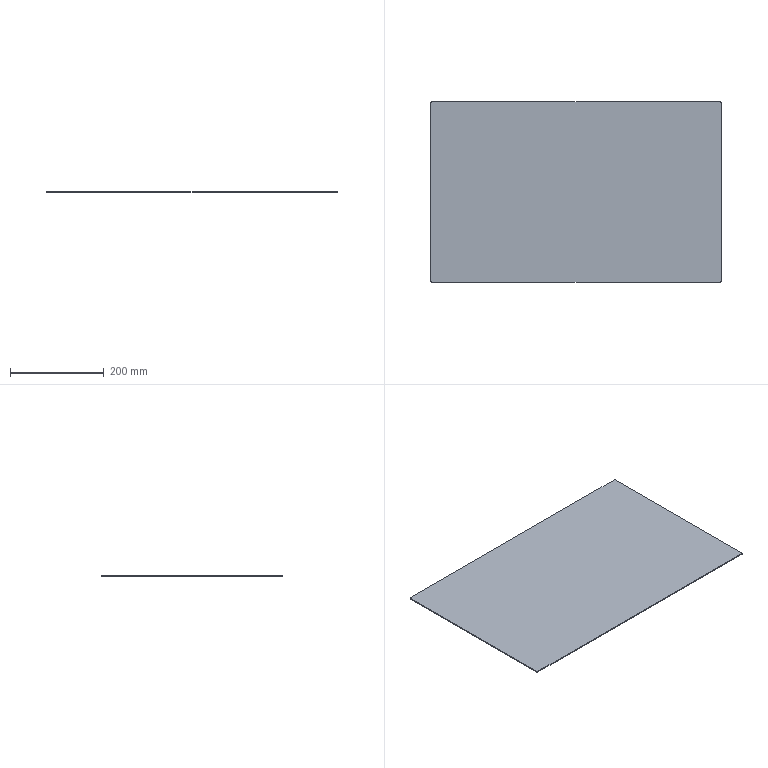Part | STEP file | Kanban base plate | 1 solid | 10 faces | box 620 x 386 x 2 mm | volume 478633 mm3 | plane 6 | cylinder 4 | commonest cylinder face diameters 4 x4
STEP:
#1=CARTESIAN_POINT('',(0.,0.,0.));
#2=DIRECTION('',(0.,0.,1.));
#3=DIRECTION('',(1.,0.,0.));
#4=AXIS2_PLACEMENT_3D('',#1,#2,#3);
#5=CARTESIAN_POINT('',(310.,-191.,2.));
#6=VERTEX_POINT('',#5);
#7=CARTESIAN_POINT('',(310.,191.,2.));
#8=VERTEX_POINT('',#7);
#9=CARTESIAN_POINT('',(310.,193.,2.));
#10=DIRECTION('',(0.,1.,0.));
#11=VECTOR('',#10,1.);
#12=LINE('',#9,#11);
#13=CARTESIAN_POINT('',(310.,193.,2.));
#14=DIRECTION('',(-1.,0.,0.));
#15=DIRECTION('',(0.,0.,1.));
#16=AXIS2_PLACEMENT_3D('',#13,#14,#15);
#17=PLANE('',#16);
#18=CARTESIAN_POINT('',(0.,0.));
#19=DIRECTION('',(0.,1.));
#20=VECTOR('',#19,1.);
#21=LINE('',#18,#20);
#22=(GEOMETRIC_REPRESENTATION_CONTEXT(2)PARAMETRIC_REPRESENTATION_CONTEXT()REPRESENTATION_CONTEXT('',''));
#23=DEFINITIONAL_REPRESENTATION('',(#21),#22);
#24=PCURVE('',#17,#23);
#25=CARTESIAN_POINT('',(0.,0.,2.));
#26=DIRECTION('',(0.,0.,1.));
#27=DIRECTION('',(1.,0.,0.));
#28=AXIS2_PLACEMENT_3D('',#25,#26,#27);
#29=PLANE('',#28);
#30=CARTESIAN_POINT('',(310.,193.));
#31=DIRECTION('',(0.,1.));
#32=VECTOR('',#31,1.);
#33=LINE('',#30,#32);
#34=(GEOMETRIC_REPRESENTATION_CONTEXT(2)PARAMETRIC_REPRESENTATION_CONTEXT()REPRESENTATION_CONTEXT('',''));
#35=DEFINITIONAL_REPRESENTATION('',(#33),#34);
#36=PCURVE('',#29,#35);
#37=SURFACE_CURVE('',#12,(#24,#36),.PCURVE_S1.);
#38=EDGE_CURVE('',#6,#8,#37,.T.);
#39=ORIENTED_EDGE('',*,*,#38,.F.);
#40=CARTESIAN_POINT('',(310.,-191.,0.));
#41=VERTEX_POINT('',#40);
#42=CARTESIAN_POINT('',(310.,-191.,2.));
#43=DIRECTION('',(0.,0.,-1.));
#44=VECTOR('',#43,1.);
#45=LINE('',#42,#44);
#46=CARTESIAN_POINT('',(0.,-384.));
#47=DIRECTION('',(-1.,0.));
#48=VECTOR('',#47,1.);
#49=LINE('',#46,#48);
#50=(GEOMETRIC_REPRESENTATION_CONTEXT(2)PARAMETRIC_REPRESENTATION_CONTEXT()REPRESENTATION_CONTEXT('',''));
#51=DEFINITIONAL_REPRESENTATION('',(#49),#50);
#52=PCURVE('',#17,#51);
#53=CARTESIAN_POINT('',(308.,-191.,2.));
#54=DIRECTION('',(0.,0.,-1.));
#55=DIRECTION('',(-1.,0.,0.));
#56=AXIS2_PLACEMENT_3D('',#53,#54,#55);
#57=CYLINDRICAL_SURFACE('',#56,2.);
#58=CARTESIAN_POINT('',(3.142,0.));
#59=DIRECTION('',(0.,1.));
#60=VECTOR('',#59,1.);
#61=LINE('',#58,#60);
#62=(GEOMETRIC_REPRESENTATION_CONTEXT(2)PARAMETRIC_REPRESENTATION_CONTEXT()REPRESENTATION_CONTEXT('',''));
#63=DEFINITIONAL_REPRESENTATION('',(#61),#62);
#64=PCURVE('',#57,#63);
#65=SURFACE_CURVE('',#45,(#52,#64),.PCURVE_S1.);
#66=EDGE_CURVE('',#6,#41,#65,.T.);
#67=ORIENTED_EDGE('',*,*,#66,.T.);
#68=CARTESIAN_POINT('',(310.,191.,0.));
#69=VERTEX_POINT('',#68);
#70=CARTESIAN_POINT('',(310.,193.,0.));
#71=DIRECTION('',(0.,1.,0.));
#72=VECTOR('',#71,1.);
#73=LINE('',#70,#72);
#74=CARTESIAN_POINT('',(-2.,0.));
#75=DIRECTION('',(0.,1.));
#76=VECTOR('',#75,1.);
#77=LINE('',#74,#76);
#78=(GEOMETRIC_REPRESENTATION_CONTEXT(2)PARAMETRIC_REPRESENTATION_CONTEXT()REPRESENTATION_CONTEXT('',''));
#79=DEFINITIONAL_REPRESENTATION('',(#77),#78);
#80=PCURVE('',#17,#79);
#81=CARTESIAN_POINT('',(0.,0.,0.));
#82=DIRECTION('',(0.,0.,1.));
#83=DIRECTION('',(1.,0.,0.));
#84=AXIS2_PLACEMENT_3D('',#81,#82,#83);
#85=PLANE('',#84);
#86=CARTESIAN_POINT('',(310.,193.));
#87=DIRECTION('',(0.,1.));
#88=VECTOR('',#87,1.);
#89=LINE('',#86,#88);
#90=(GEOMETRIC_REPRESENTATION_CONTEXT(2)PARAMETRIC_REPRESENTATION_CONTEXT()REPRESENTATION_CONTEXT('',''));
#91=DEFINITIONAL_REPRESENTATION('',(#89),#90);
#92=PCURVE('',#85,#91);
#93=SURFACE_CURVE('',#73,(#80,#92),.PCURVE_S1.);
#94=EDGE_CURVE('',#41,#69,#93,.T.);
#95=ORIENTED_EDGE('',*,*,#94,.T.);
#96=CARTESIAN_POINT('',(310.,191.,2.));
#97=DIRECTION('',(0.,0.,1.));
#98=VECTOR('',#97,1.);
#99=LINE('',#96,#98);
#100=CARTESIAN_POINT('',(0.,-2.));
#101=DIRECTION('',(1.,0.));
#102=VECTOR('',#101,1.);
#103=LINE('',#100,#102);
#104=(GEOMETRIC_REPRESENTATION_CONTEXT(2)PARAMETRIC_REPRESENTATION_CONTEXT()REPRESENTATION_CONTEXT('',''));
#105=DEFINITIONAL_REPRESENTATION('',(#103),#104);
#106=PCURVE('',#17,#105);
#107=CARTESIAN_POINT('',(308.,191.,2.));
#108=DIRECTION('',(0.,0.,-1.));
#109=DIRECTION('',(-1.,0.,0.));
#110=AXIS2_PLACEMENT_3D('',#107,#108,#109);
#111=CYLINDRICAL_SURFACE('',#110,2.);
#112=CARTESIAN_POINT('',(3.142,0.));
#113=DIRECTION('',(0.,-1.));
#114=VECTOR('',#113,1.);
#115=LINE('',#112,#114);
#116=(GEOMETRIC_REPRESENTATION_CONTEXT(2)PARAMETRIC_REPRESENTATION_CONTEXT()REPRESENTATION_CONTEXT('',''));
#117=DEFINITIONAL_REPRESENTATION('',(#115),#116);
#118=PCURVE('',#111,#117);
#119=SURFACE_CURVE('',#99,(#106,#118),.PCURVE_S1.);
#120=EDGE_CURVE('',#69,#8,#119,.T.);
#121=ORIENTED_EDGE('',*,*,#120,.T.);
#122=EDGE_LOOP('',(#39,#67,#95,#121));
#123=FACE_BOUND('',#122,.T.);
#124=ADVANCED_FACE('',(#123),#17,.F.);
#125=CARTESIAN_POINT('',(308.,193.,2.));
#126=VERTEX_POINT('',#125);
#127=CARTESIAN_POINT('',(-308.,193.,2.));
#128=VERTEX_POINT('',#127);
#129=CARTESIAN_POINT('',(-310.,193.,2.));
#130=DIRECTION('',(-1.,0.,0.));
#131=VECTOR('',#130,1.);
#132=LINE('',#129,#131);
#133=CARTESIAN_POINT('',(-310.,193.,2.));
#134=DIRECTION('',(0.,-1.,0.));
#135=DIRECTION('',(0.,0.,-1.));
#136=AXIS2_PLACEMENT_3D('',#133,#134,#135);
#137=PLANE('',#136);
#138=CARTESIAN_POINT('',(0.,0.));
#139=DIRECTION('',(0.,-1.));
#140=VECTOR('',#139,1.);
#141=LINE('',#138,#140);
#142=(GEOMETRIC_REPRESENTATION_CONTEXT(2)PARAMETRIC_REPRESENTATION_CONTEXT()REPRESENTATION_CONTEXT('',''));
#143=DEFINITIONAL_REPRESENTATION('',(#141),#142);
#144=PCURVE('',#137,#143);
#145=CARTESIAN_POINT('',(-310.,193.));
#146=DIRECTION('',(-1.,0.));
#147=VECTOR('',#146,1.);
#148=LINE('',#145,#147);
#149=(GEOMETRIC_REPRESENTATION_CONTEXT(2)PARAMETRIC_REPRESENTATION_CONTEXT()REPRESENTATION_CONTEXT('',''));
#150=DEFINITIONAL_REPRESENTATION('',(#148),#149);
#151=PCURVE('',#29,#150);
#152=SURFACE_CURVE('',#132,(#144,#151),.PCURVE_S1.);
#153=EDGE_CURVE('',#126,#128,#152,.T.);
#154=ORIENTED_EDGE('',*,*,#153,.F.);
#155=CARTESIAN_POINT('',(308.,193.,0.));
#156=VERTEX_POINT('',#155);
#157=CARTESIAN_POINT('',(308.,193.,2.));
#158=DIRECTION('',(0.,0.,-1.));
#159=VECTOR('',#158,1.);
#160=LINE('',#157,#159);
#161=CARTESIAN_POINT('',(0.,618.));
#162=DIRECTION('',(1.,0.));
#163=VECTOR('',#162,1.);
#164=LINE('',#161,#163);
#165=(GEOMETRIC_REPRESENTATION_CONTEXT(2)PARAMETRIC_REPRESENTATION_CONTEXT()REPRESENTATION_CONTEXT('',''));
#166=DEFINITIONAL_REPRESENTATION('',(#164),#165);
#167=PCURVE('',#137,#166);
#168=CARTESIAN_POINT('',(1.571,0.));
#169=DIRECTION('',(0.,1.));
#170=VECTOR('',#169,1.);
#171=LINE('',#168,#170);
#172=(GEOMETRIC_REPRESENTATION_CONTEXT(2)PARAMETRIC_REPRESENTATION_CONTEXT()REPRESENTATION_CONTEXT('',''));
#173=DEFINITIONAL_REPRESENTATION('',(#171),#172);
#174=PCURVE('',#111,#173);
#175=SURFACE_CURVE('',#160,(#167,#174),.PCURVE_S1.);
#176=EDGE_CURVE('',#126,#156,#175,.T.);
#177=ORIENTED_EDGE('',*,*,#176,.T.);
#178=CARTESIAN_POINT('',(-308.,193.,0.));
#179=VERTEX_POINT('',#178);
#180=CARTESIAN_POINT('',(-310.,193.,0.));
#181=DIRECTION('',(-1.,0.,0.));
#182=VECTOR('',#181,1.);
#183=LINE('',#180,#182);
#184=CARTESIAN_POINT('',(2.,0.));
#185=DIRECTION('',(0.,-1.));
#186=VECTOR('',#185,1.);
#187=LINE('',#184,#186);
#188=(GEOMETRIC_REPRESENTATION_CONTEXT(2)PARAMETRIC_REPRESENTATION_CONTEXT()REPRESENTATION_CONTEXT('',''));
#189=DEFINITIONAL_REPRESENTATION('',(#187),#188);
#190=PCURVE('',#137,#189);
#191=CARTESIAN_POINT('',(-310.,193.));
#192=DIRECTION('',(-1.,0.));
#193=VECTOR('',#192,1.);
#194=LINE('',#191,#193);
#195=(GEOMETRIC_REPRESENTATION_CONTEXT(2)PARAMETRIC_REPRESENTATION_CONTEXT()REPRESENTATION_CONTEXT('',''));
#196=DEFINITIONAL_REPRESENTATION('',(#194),#195);
#197=PCURVE('',#85,#196);
#198=SURFACE_CURVE('',#183,(#190,#197),.PCURVE_S1.);
#199=EDGE_CURVE('',#156,#179,#198,.T.);
#200=ORIENTED_EDGE('',*,*,#199,.T.);
#201=CARTESIAN_POINT('',(-308.,193.,2.));
#202=DIRECTION('',(0.,0.,1.));
#203=VECTOR('',#202,1.);
#204=LINE('',#201,#203);
#205=CARTESIAN_POINT('',(0.,2.));
#206=DIRECTION('',(-1.,0.));
#207=VECTOR('',#206,1.);
#208=LINE('',#205,#207);
#209=(GEOMETRIC_REPRESENTATION_CONTEXT(2)PARAMETRIC_REPRESENTATION_CONTEXT()REPRESENTATION_CONTEXT('',''));
#210=DEFINITIONAL_REPRESENTATION('',(#208),#209);
#211=PCURVE('',#137,#210);
#212=CARTESIAN_POINT('',(-308.,191.,2.));
#213=DIRECTION('',(0.,0.,-1.));
#214=DIRECTION('',(-1.,0.,0.));
#215=AXIS2_PLACEMENT_3D('',#212,#213,#214);
#216=CYLINDRICAL_SURFACE('',#215,2.);
#217=CARTESIAN_POINT('',(1.571,0.));
#218=DIRECTION('',(0.,-1.));
#219=VECTOR('',#218,1.);
#220=LINE('',#217,#219);
#221=(GEOMETRIC_REPRESENTATION_CONTEXT(2)PARAMETRIC_REPRESENTATION_CONTEXT()REPRESENTATION_CONTEXT('',''));
#222=DEFINITIONAL_REPRESENTATION('',(#220),#221);
#223=PCURVE('',#216,#222);
#224=SURFACE_CURVE('',#204,(#211,#223),.PCURVE_S1.);
#225=EDGE_CURVE('',#179,#128,#224,.T.);
#226=ORIENTED_EDGE('',*,*,#225,.T.);
#227=EDGE_LOOP('',(#154,#177,#200,#226));
#228=FACE_BOUND('',#227,.T.);
#229=ADVANCED_FACE('',(#228),#137,.F.);
#230=CARTESIAN_POINT('',(-310.,191.,0.));
#231=VERTEX_POINT('',#230);
#232=CARTESIAN_POINT('',(-310.,-191.,0.));
#233=VERTEX_POINT('',#232);
#234=CARTESIAN_POINT('',(-310.,193.,0.));
#235=DIRECTION('',(0.,-1.,0.));
#236=VECTOR('',#235,1.);
#237=LINE('',#234,#236);
#238=CARTESIAN_POINT('',(-310.,193.,2.));
#239=DIRECTION('',(1.,0.,0.));
#240=DIRECTION('',(0.,0.,-1.));
#241=AXIS2_PLACEMENT_3D('',#238,#239,#240);
#242=PLANE('',#241);
#243=CARTESIAN_POINT('',(2.,0.));
#244=DIRECTION('',(0.,-1.));
#245=VECTOR('',#244,1.);
#246=LINE('',#243,#245);
#247=(GEOMETRIC_REPRESENTATION_CONTEXT(2)PARAMETRIC_REPRESENTATION_CONTEXT()REPRESENTATION_CONTEXT('',''));
#248=DEFINITIONAL_REPRESENTATION('',(#246),#247);
#249=PCURVE('',#242,#248);
#250=CARTESIAN_POINT('',(-310.,193.));
#251=DIRECTION('',(0.,-1.));
#252=VECTOR('',#251,1.);
#253=LINE('',#250,#252);
#254=(GEOMETRIC_REPRESENTATION_CONTEXT(2)PARAMETRIC_REPRESENTATION_CONTEXT()REPRESENTATION_CONTEXT('',''));
#255=DEFINITIONAL_REPRESENTATION('',(#253),#254);
#256=PCURVE('',#85,#255);
#257=SURFACE_CURVE('',#237,(#249,#256),.PCURVE_S1.);
#258=EDGE_CURVE('',#231,#233,#257,.T.);
#259=ORIENTED_EDGE('',*,*,#258,.T.);
#260=CARTESIAN_POINT('',(-310.,-191.,2.));
#261=VERTEX_POINT('',#260);
#262=CARTESIAN_POINT('',(-310.,-191.,2.));
#263=DIRECTION('',(0.,0.,1.));
#264=VECTOR('',#263,1.);
#265=LINE('',#262,#264);
#266=CARTESIAN_POINT('',(0.,-384.));
#267=DIRECTION('',(-1.,0.));
#268=VECTOR('',#267,1.);
#269=LINE('',#266,#268);
#270=(GEOMETRIC_REPRESENTATION_CONTEXT(2)PARAMETRIC_REPRESENTATION_CONTEXT()REPRESENTATION_CONTEXT('',''));
#271=DEFINITIONAL_REPRESENTATION('',(#269),#270);
#272=PCURVE('',#242,#271);
#273=CARTESIAN_POINT('',(-308.,-191.,2.));
#274=DIRECTION('',(0.,0.,-1.));
#275=DIRECTION('',(-1.,0.,0.));
#276=AXIS2_PLACEMENT_3D('',#273,#274,#275);
#277=CYLINDRICAL_SURFACE('',#276,2.);
#278=CARTESIAN_POINT('',(6.283,0.));
#279=DIRECTION('',(0.,-1.));
#280=VECTOR('',#279,1.);
#281=LINE('',#278,#280);
#282=(GEOMETRIC_REPRESENTATION_CONTEXT(2)PARAMETRIC_REPRESENTATION_CONTEXT()REPRESENTATION_CONTEXT('',''));
#283=DEFINITIONAL_REPRESENTATION('',(#281),#282);
#284=PCURVE('',#277,#283);
#285=SURFACE_CURVE('',#265,(#272,#284),.PCURVE_S1.);
#286=EDGE_CURVE('',#233,#261,#285,.T.);
#287=ORIENTED_EDGE('',*,*,#286,.T.);
#288=CARTESIAN_POINT('',(-310.,191.,2.));
#289=VERTEX_POINT('',#288);
#290=CARTESIAN_POINT('',(-310.,193.,2.));
#291=DIRECTION('',(0.,-1.,0.));
#292=VECTOR('',#291,1.);
#293=LINE('',#290,#292);
#294=CARTESIAN_POINT('',(0.,0.));
#295=DIRECTION('',(0.,-1.));
#296=VECTOR('',#295,1.);
#297=LINE('',#294,#296);
#298=(GEOMETRIC_REPRESENTATION_CONTEXT(2)PARAMETRIC_REPRESENTATION_CONTEXT()REPRESENTATION_CONTEXT('',''));
#299=DEFINITIONAL_REPRESENTATION('',(#297),#298);
#300=PCURVE('',#242,#299);
#301=CARTESIAN_POINT('',(-310.,193.));
#302=DIRECTION('',(0.,-1.));
#303=VECTOR('',#302,1.);
#304=LINE('',#301,#303);
#305=(GEOMETRIC_REPRESENTATION_CONTEXT(2)PARAMETRIC_REPRESENTATION_CONTEXT()REPRESENTATION_CONTEXT('',''));
#306=DEFINITIONAL_REPRESENTATION('',(#304),#305);
#307=PCURVE('',#29,#306);
#308=SURFACE_CURVE('',#293,(#300,#307),.PCURVE_S1.);
#309=EDGE_CURVE('',#289,#261,#308,.T.);
#310=ORIENTED_EDGE('',*,*,#309,.F.);
#311=CARTESIAN_POINT('',(-310.,191.,2.));
#312=DIRECTION('',(0.,0.,-1.));
#313=VECTOR('',#312,1.);
#314=LINE('',#311,#313);
#315=CARTESIAN_POINT('',(0.,-2.));
#316=DIRECTION('',(1.,0.));
#317=VECTOR('',#316,1.);
#318=LINE('',#315,#317);
#319=(GEOMETRIC_REPRESENTATION_CONTEXT(2)PARAMETRIC_REPRESENTATION_CONTEXT()REPRESENTATION_CONTEXT('',''));
#320=DEFINITIONAL_REPRESENTATION('',(#318),#319);
#321=PCURVE('',#242,#320);
#322=CARTESIAN_POINT('',(0.,0.));
#323=DIRECTION('',(0.,1.));
#324=VECTOR('',#323,1.);
#325=LINE('',#322,#324);
#326=(GEOMETRIC_REPRESENTATION_CONTEXT(2)PARAMETRIC_REPRESENTATION_CONTEXT()REPRESENTATION_CONTEXT('',''));
#327=DEFINITIONAL_REPRESENTATION('',(#325),#326);
#328=PCURVE('',#216,#327);
#329=SURFACE_CURVE('',#314,(#321,#328),.PCURVE_S1.);
#330=EDGE_CURVE('',#289,#231,#329,.T.);
#331=ORIENTED_EDGE('',*,*,#330,.T.);
#332=EDGE_LOOP('',(#259,#287,#310,#331));
#333=FACE_BOUND('',#332,.T.);
#334=ADVANCED_FACE('',(#333),#242,.F.);
#335=CARTESIAN_POINT('',(-308.,-193.,0.));
#336=VERTEX_POINT('',#335);
#337=CARTESIAN_POINT('',(308.,-193.,0.));
#338=VERTEX_POINT('',#337);
#339=CARTESIAN_POINT('',(-310.,-193.,0.));
#340=DIRECTION('',(1.,0.,0.));
#341=VECTOR('',#340,1.);
#342=LINE('',#339,#341);
#343=CARTESIAN_POINT('',(-310.,-193.,2.));
#344=DIRECTION('',(0.,1.,0.));
#345=DIRECTION('',(0.,0.,1.));
#346=AXIS2_PLACEMENT_3D('',#343,#344,#345);
#347=PLANE('',#346);
#348=CARTESIAN_POINT('',(-2.,0.));
#349=DIRECTION('',(0.,1.));
#350=VECTOR('',#349,1.);
#351=LINE('',#348,#350);
#352=(GEOMETRIC_REPRESENTATION_CONTEXT(2)PARAMETRIC_REPRESENTATION_CONTEXT()REPRESENTATION_CONTEXT('',''));
#353=DEFINITIONAL_REPRESENTATION('',(#351),#352);
#354=PCURVE('',#347,#353);
#355=CARTESIAN_POINT('',(-310.,-193.));
#356=DIRECTION('',(1.,0.));
#357=VECTOR('',#356,1.);
#358=LINE('',#355,#357);
#359=(GEOMETRIC_REPRESENTATION_CONTEXT(2)PARAMETRIC_REPRESENTATION_CONTEXT()REPRESENTATION_CONTEXT('',''));
#360=DEFINITIONAL_REPRESENTATION('',(#358),#359);
#361=PCURVE('',#85,#360);
#362=SURFACE_CURVE('',#342,(#354,#361),.PCURVE_S1.);
#363=EDGE_CURVE('',#336,#338,#362,.T.);
#364=ORIENTED_EDGE('',*,*,#363,.T.);
#365=CARTESIAN_POINT('',(308.,-193.,2.));
#366=VERTEX_POINT('',#365);
#367=CARTESIAN_POINT('',(308.,-193.,2.));
#368=DIRECTION('',(0.,0.,1.));
#369=VECTOR('',#368,1.);
#370=LINE('',#367,#369);
#371=CARTESIAN_POINT('',(0.,618.));
#372=DIRECTION('',(1.,0.));
#373=VECTOR('',#372,1.);
#374=LINE('',#371,#373);
#375=(GEOMETRIC_REPRESENTATION_CONTEXT(2)PARAMETRIC_REPRESENTATION_CONTEXT()REPRESENTATION_CONTEXT('',''));
#376=DEFINITIONAL_REPRESENTATION('',(#374),#375);
#377=PCURVE('',#347,#376);
#378=CARTESIAN_POINT('',(4.712,0.));
#379=DIRECTION('',(0.,-1.));
#380=VECTOR('',#379,1.);
#381=LINE('',#378,#380);
#382=(GEOMETRIC_REPRESENTATION_CONTEXT(2)PARAMETRIC_REPRESENTATION_CONTEXT()REPRESENTATION_CONTEXT('',''));
#383=DEFINITIONAL_REPRESENTATION('',(#381),#382);
#384=PCURVE('',#57,#383);
#385=SURFACE_CURVE('',#370,(#377,#384),.PCURVE_S1.);
#386=EDGE_CURVE('',#338,#366,#385,.T.);
#387=ORIENTED_EDGE('',*,*,#386,.T.);
#388=CARTESIAN_POINT('',(-308.,-193.,2.));
#389=VERTEX_POINT('',#388);
#390=CARTESIAN_POINT('',(-310.,-193.,2.));
#391=DIRECTION('',(1.,0.,0.));
#392=VECTOR('',#391,1.);
#393=LINE('',#390,#392);
#394=CARTESIAN_POINT('',(0.,0.));
#395=DIRECTION('',(0.,1.));
#396=VECTOR('',#395,1.);
#397=LINE('',#394,#396);
#398=(GEOMETRIC_REPRESENTATION_CONTEXT(2)PARAMETRIC_REPRESENTATION_CONTEXT()REPRESENTATION_CONTEXT('',''));
#399=DEFINITIONAL_REPRESENTATION('',(#397),#398);
#400=PCURVE('',#347,#399);
#401=CARTESIAN_POINT('',(-310.,-193.));
#402=DIRECTION('',(1.,0.));
#403=VECTOR('',#402,1.);
#404=LINE('',#401,#403);
#405=(GEOMETRIC_REPRESENTATION_CONTEXT(2)PARAMETRIC_REPRESENTATION_CONTEXT()REPRESENTATION_CONTEXT('',''));
#406=DEFINITIONAL_REPRESENTATION('',(#404),#405);
#407=PCURVE('',#29,#406);
#408=SURFACE_CURVE('',#393,(#400,#407),.PCURVE_S1.);
#409=EDGE_CURVE('',#389,#366,#408,.T.);
#410=ORIENTED_EDGE('',*,*,#409,.F.);
#411=CARTESIAN_POINT('',(-308.,-193.,2.));
#412=DIRECTION('',(0.,0.,-1.));
#413=VECTOR('',#412,1.);
#414=LINE('',#411,#413);
#415=CARTESIAN_POINT('',(0.,2.));
#416=DIRECTION('',(-1.,0.));
#417=VECTOR('',#416,1.);
#418=LINE('',#415,#417);
#419=(GEOMETRIC_REPRESENTATION_CONTEXT(2)PARAMETRIC_REPRESENTATION_CONTEXT()REPRESENTATION_CONTEXT('',''));
#420=DEFINITIONAL_REPRESENTATION('',(#418),#419);
#421=PCURVE('',#347,#420);
#422=CARTESIAN_POINT('',(4.712,0.));
#423=DIRECTION('',(0.,1.));
#424=VECTOR('',#423,1.);
#425=LINE('',#422,#424);
#426=(GEOMETRIC_REPRESENTATION_CONTEXT(2)PARAMETRIC_REPRESENTATION_CONTEXT()REPRESENTATION_CONTEXT('',''));
#427=DEFINITIONAL_REPRESENTATION('',(#425),#426);
#428=PCURVE('',#277,#427);
#429=SURFACE_CURVE('',#414,(#421,#428),.PCURVE_S1.);
#430=EDGE_CURVE('',#389,#336,#429,.T.);
#431=ORIENTED_EDGE('',*,*,#430,.T.);
#432=EDGE_LOOP('',(#364,#387,#410,#431));
#433=FACE_BOUND('',#432,.T.);
#434=ADVANCED_FACE('',(#433),#347,.F.);
#435=ORIENTED_EDGE('',*,*,#409,.T.);
#436=CARTESIAN_POINT('',(308.,-191.,2.));
#437=DIRECTION('',(0.,0.,1.));
#438=DIRECTION('',(1.,0.,0.));
#439=AXIS2_PLACEMENT_3D('',#436,#437,#438);
#440=CIRCLE('',#439,2.);
#441=CARTESIAN_POINT('',(308.,-191.));
#442=DIRECTION('',(1.,0.));
#443=AXIS2_PLACEMENT_2D('',#441,#442);
#444=CIRCLE('',#443,2.);
#445=(GEOMETRIC_REPRESENTATION_CONTEXT(2)PARAMETRIC_REPRESENTATION_CONTEXT()REPRESENTATION_CONTEXT('',''));
#446=DEFINITIONAL_REPRESENTATION('',(#444),#445);
#447=PCURVE('',#29,#446);
#448=CARTESIAN_POINT('',(9.425,0.));
#449=DIRECTION('',(-1.,0.));
#450=VECTOR('',#449,1.);
#451=LINE('',#448,#450);
#452=(GEOMETRIC_REPRESENTATION_CONTEXT(2)PARAMETRIC_REPRESENTATION_CONTEXT()REPRESENTATION_CONTEXT('',''));
#453=DEFINITIONAL_REPRESENTATION('',(#451),#452);
#454=PCURVE('',#57,#453);
#455=SURFACE_CURVE('',#440,(#447,#454),.PCURVE_S1.);
#456=EDGE_CURVE('',#366,#6,#455,.T.);
#457=ORIENTED_EDGE('',*,*,#456,.T.);
#458=ORIENTED_EDGE('',*,*,#38,.T.);
#459=CARTESIAN_POINT('',(308.,191.,2.));
#460=DIRECTION('',(0.,0.,1.));
#461=DIRECTION('',(1.,0.,0.));
#462=AXIS2_PLACEMENT_3D('',#459,#460,#461);
#463=CIRCLE('',#462,2.);
#464=CARTESIAN_POINT('',(308.,191.));
#465=DIRECTION('',(1.,0.));
#466=AXIS2_PLACEMENT_2D('',#464,#465);
#467=CIRCLE('',#466,2.);
#468=(GEOMETRIC_REPRESENTATION_CONTEXT(2)PARAMETRIC_REPRESENTATION_CONTEXT()REPRESENTATION_CONTEXT('',''));
#469=DEFINITIONAL_REPRESENTATION('',(#467),#468);
#470=PCURVE('',#29,#469);
#471=CARTESIAN_POINT('',(3.142,0.));
#472=DIRECTION('',(-1.,0.));
#473=VECTOR('',#472,1.);
#474=LINE('',#471,#473);
#475=(GEOMETRIC_REPRESENTATION_CONTEXT(2)PARAMETRIC_REPRESENTATION_CONTEXT()REPRESENTATION_CONTEXT('',''));
#476=DEFINITIONAL_REPRESENTATION('',(#474),#475);
#477=PCURVE('',#111,#476);
#478=SURFACE_CURVE('',#463,(#470,#477),.PCURVE_S1.);
#479=EDGE_CURVE('',#8,#126,#478,.T.);
#480=ORIENTED_EDGE('',*,*,#479,.T.);
#481=ORIENTED_EDGE('',*,*,#153,.T.);
#482=CARTESIAN_POINT('',(-308.,191.,2.));
#483=DIRECTION('',(0.,0.,1.));
#484=DIRECTION('',(1.,0.,0.));
#485=AXIS2_PLACEMENT_3D('',#482,#483,#484);
#486=CIRCLE('',#485,2.);
#487=CARTESIAN_POINT('',(-308.,191.));
#488=DIRECTION('',(1.,0.));
#489=AXIS2_PLACEMENT_2D('',#487,#488);
#490=CIRCLE('',#489,2.);
#491=(GEOMETRIC_REPRESENTATION_CONTEXT(2)PARAMETRIC_REPRESENTATION_CONTEXT()REPRESENTATION_CONTEXT('',''));
#492=DEFINITIONAL_REPRESENTATION('',(#490),#491);
#493=PCURVE('',#29,#492);
#494=CARTESIAN_POINT('',(3.142,0.));
#495=DIRECTION('',(-1.,0.));
#496=VECTOR('',#495,1.);
#497=LINE('',#494,#496);
#498=(GEOMETRIC_REPRESENTATION_CONTEXT(2)PARAMETRIC_REPRESENTATION_CONTEXT()REPRESENTATION_CONTEXT('',''));
#499=DEFINITIONAL_REPRESENTATION('',(#497),#498);
#500=PCURVE('',#216,#499);
#501=SURFACE_CURVE('',#486,(#493,#500),.PCURVE_S1.);
#502=EDGE_CURVE('',#128,#289,#501,.T.);
#503=ORIENTED_EDGE('',*,*,#502,.T.);
#504=ORIENTED_EDGE('',*,*,#309,.T.);
#505=CARTESIAN_POINT('',(-308.,-191.,2.));
#506=DIRECTION('',(0.,0.,1.));
#507=DIRECTION('',(1.,0.,0.));
#508=AXIS2_PLACEMENT_3D('',#505,#506,#507);
#509=CIRCLE('',#508,2.);
#510=CARTESIAN_POINT('',(-308.,-191.));
#511=DIRECTION('',(1.,0.));
#512=AXIS2_PLACEMENT_2D('',#510,#511);
#513=CIRCLE('',#512,2.);
#514=(GEOMETRIC_REPRESENTATION_CONTEXT(2)PARAMETRIC_REPRESENTATION_CONTEXT()REPRESENTATION_CONTEXT('',''));
#515=DEFINITIONAL_REPRESENTATION('',(#513),#514);
#516=PCURVE('',#29,#515);
#517=CARTESIAN_POINT('',(9.425,0.));
#518=DIRECTION('',(-1.,0.));
#519=VECTOR('',#518,1.);
#520=LINE('',#517,#519);
#521=(GEOMETRIC_REPRESENTATION_CONTEXT(2)PARAMETRIC_REPRESENTATION_CONTEXT()REPRESENTATION_CONTEXT('',''));
#522=DEFINITIONAL_REPRESENTATION('',(#520),#521);
#523=PCURVE('',#277,#522);
#524=SURFACE_CURVE('',#509,(#516,#523),.PCURVE_S1.);
#525=EDGE_CURVE('',#261,#389,#524,.T.);
#526=ORIENTED_EDGE('',*,*,#525,.T.);
#527=EDGE_LOOP('',(#435,#457,#458,#480,#481,#503,#504,#526));
#528=FACE_BOUND('',#527,.T.);
#529=ADVANCED_FACE('',(#528),#29,.T.);
#530=ORIENTED_EDGE('',*,*,#94,.F.);
#531=CARTESIAN_POINT('',(308.,-191.,0.));
#532=DIRECTION('',(0.,0.,-1.));
#533=DIRECTION('',(1.,0.,0.));
#534=AXIS2_PLACEMENT_3D('',#531,#532,#533);
#535=CIRCLE('',#534,2.);
#536=CARTESIAN_POINT('',(310.,-191.));
#537=CARTESIAN_POINT('',(310.,-194.464));
#538=CARTESIAN_POINT('',(307.,-192.732));
#539=CARTESIAN_POINT('',(304.,-191.));
#540=CARTESIAN_POINT('',(307.,-189.268));
#541=CARTESIAN_POINT('',(310.,-187.536));
#542=CARTESIAN_POINT('',(310.,-191.));
#543=(BOUNDED_CURVE()B_SPLINE_CURVE(2,(#536,#537,#538,#539,#540,#541,#542),.UNSPECIFIED.,.T.,.F.)B_SPLINE_CURVE_WITH_KNOTS((1,2,2,2,2,1),(-2.094,0.,2.094,4.189,6.283,8.378),.UNSPECIFIED.)CURVE()GEOMETRIC_REPRESENTATION_ITEM()RATIONAL_B_SPLINE_CURVE((1.,0.5,1.,0.5,1.,0.5,1.))REPRESENTATION_ITEM(''));
#544=(GEOMETRIC_REPRESENTATION_CONTEXT(2)PARAMETRIC_REPRESENTATION_CONTEXT()REPRESENTATION_CONTEXT('',''));
#545=DEFINITIONAL_REPRESENTATION('',(#543),#544);
#546=PCURVE('',#85,#545);
#547=CARTESIAN_POINT('',(3.142,2.));
#548=DIRECTION('',(1.,0.));
#549=VECTOR('',#548,1.);
#550=LINE('',#547,#549);
#551=(GEOMETRIC_REPRESENTATION_CONTEXT(2)PARAMETRIC_REPRESENTATION_CONTEXT()REPRESENTATION_CONTEXT('',''));
#552=DEFINITIONAL_REPRESENTATION('',(#550),#551);
#553=PCURVE('',#57,#552);
#554=SURFACE_CURVE('',#535,(#546,#553),.PCURVE_S1.);
#555=EDGE_CURVE('',#41,#338,#554,.T.);
#556=ORIENTED_EDGE('',*,*,#555,.T.);
#557=ORIENTED_EDGE('',*,*,#363,.F.);
#558=CARTESIAN_POINT('',(-308.,-191.,0.));
#559=DIRECTION('',(0.,0.,-1.));
#560=DIRECTION('',(1.,0.,0.));
#561=AXIS2_PLACEMENT_3D('',#558,#559,#560);
#562=CIRCLE('',#561,2.);
#563=CARTESIAN_POINT('',(-306.,-191.));
#564=CARTESIAN_POINT('',(-306.,-194.464));
#565=CARTESIAN_POINT('',(-309.,-192.732));
#566=CARTESIAN_POINT('',(-312.,-191.));
#567=CARTESIAN_POINT('',(-309.,-189.268));
#568=CARTESIAN_POINT('',(-306.,-187.536));
#569=CARTESIAN_POINT('',(-306.,-191.));
#570=(BOUNDED_CURVE()B_SPLINE_CURVE(2,(#563,#564,#565,#566,#567,#568,#569),.UNSPECIFIED.,.T.,.F.)B_SPLINE_CURVE_WITH_KNOTS((1,2,2,2,2,1),(-2.094,0.,2.094,4.189,6.283,8.378),.UNSPECIFIED.)CURVE()GEOMETRIC_REPRESENTATION_ITEM()RATIONAL_B_SPLINE_CURVE((1.,0.5,1.,0.5,1.,0.5,1.))REPRESENTATION_ITEM(''));
#571=(GEOMETRIC_REPRESENTATION_CONTEXT(2)PARAMETRIC_REPRESENTATION_CONTEXT()REPRESENTATION_CONTEXT('',''));
#572=DEFINITIONAL_REPRESENTATION('',(#570),#571);
#573=PCURVE('',#85,#572);
#574=CARTESIAN_POINT('',(3.142,2.));
#575=DIRECTION('',(1.,0.));
#576=VECTOR('',#575,1.);
#577=LINE('',#574,#576);
#578=(GEOMETRIC_REPRESENTATION_CONTEXT(2)PARAMETRIC_REPRESENTATION_CONTEXT()REPRESENTATION_CONTEXT('',''));
#579=DEFINITIONAL_REPRESENTATION('',(#577),#578);
#580=PCURVE('',#277,#579);
#581=SURFACE_CURVE('',#562,(#573,#580),.PCURVE_S1.);
#582=EDGE_CURVE('',#336,#233,#581,.T.);
#583=ORIENTED_EDGE('',*,*,#582,.T.);
#584=ORIENTED_EDGE('',*,*,#258,.F.);
#585=CARTESIAN_POINT('',(-308.,191.,0.));
#586=DIRECTION('',(0.,0.,-1.));
#587=DIRECTION('',(1.,0.,0.));
#588=AXIS2_PLACEMENT_3D('',#585,#586,#587);
#589=CIRCLE('',#588,2.);
#590=CARTESIAN_POINT('',(-306.,191.));
#591=CARTESIAN_POINT('',(-306.,187.536));
#592=CARTESIAN_POINT('',(-309.,189.268));
#593=CARTESIAN_POINT('',(-312.,191.));
#594=CARTESIAN_POINT('',(-309.,192.732));
#595=CARTESIAN_POINT('',(-306.,194.464));
#596=CARTESIAN_POINT('',(-306.,191.));
#597=(BOUNDED_CURVE()B_SPLINE_CURVE(2,(#590,#591,#592,#593,#594,#595,#596),.UNSPECIFIED.,.T.,.F.)B_SPLINE_CURVE_WITH_KNOTS((1,2,2,2,2,1),(-2.094,0.,2.094,4.189,6.283,8.378),.UNSPECIFIED.)CURVE()GEOMETRIC_REPRESENTATION_ITEM()RATIONAL_B_SPLINE_CURVE((1.,0.5,1.,0.5,1.,0.5,1.))REPRESENTATION_ITEM(''));
#598=(GEOMETRIC_REPRESENTATION_CONTEXT(2)PARAMETRIC_REPRESENTATION_CONTEXT()REPRESENTATION_CONTEXT('',''));
#599=DEFINITIONAL_REPRESENTATION('',(#597),#598);
#600=PCURVE('',#85,#599);
#601=CARTESIAN_POINT('',(-3.142,2.));
#602=DIRECTION('',(1.,0.));
#603=VECTOR('',#602,1.);
#604=LINE('',#601,#603);
#605=(GEOMETRIC_REPRESENTATION_CONTEXT(2)PARAMETRIC_REPRESENTATION_CONTEXT()REPRESENTATION_CONTEXT('',''));
#606=DEFINITIONAL_REPRESENTATION('',(#604),#605);
#607=PCURVE('',#216,#606);
#608=SURFACE_CURVE('',#589,(#600,#607),.PCURVE_S1.);
#609=EDGE_CURVE('',#231,#179,#608,.T.);
#610=ORIENTED_EDGE('',*,*,#609,.T.);
#611=ORIENTED_EDGE('',*,*,#199,.F.);
#612=CARTESIAN_POINT('',(308.,191.,0.));
#613=DIRECTION('',(0.,0.,-1.));
#614=DIRECTION('',(1.,0.,0.));
#615=AXIS2_PLACEMENT_3D('',#612,#613,#614);
#616=CIRCLE('',#615,2.);
#617=CARTESIAN_POINT('',(310.,191.));
#618=CARTESIAN_POINT('',(310.,187.536));
#619=CARTESIAN_POINT('',(307.,189.268));
#620=CARTESIAN_POINT('',(304.,191.));
#621=CARTESIAN_POINT('',(307.,192.732));
#622=CARTESIAN_POINT('',(310.,194.464));
#623=CARTESIAN_POINT('',(310.,191.));
#624=(BOUNDED_CURVE()B_SPLINE_CURVE(2,(#617,#618,#619,#620,#621,#622,#623),.UNSPECIFIED.,.T.,.F.)B_SPLINE_CURVE_WITH_KNOTS((1,2,2,2,2,1),(-2.094,0.,2.094,4.189,6.283,8.378),.UNSPECIFIED.)CURVE()GEOMETRIC_REPRESENTATION_ITEM()RATIONAL_B_SPLINE_CURVE((1.,0.5,1.,0.5,1.,0.5,1.))REPRESENTATION_ITEM(''));
#625=(GEOMETRIC_REPRESENTATION_CONTEXT(2)PARAMETRIC_REPRESENTATION_CONTEXT()REPRESENTATION_CONTEXT('',''));
#626=DEFINITIONAL_REPRESENTATION('',(#624),#625);
#627=PCURVE('',#85,#626);
#628=CARTESIAN_POINT('',(-3.142,2.));
#629=DIRECTION('',(1.,0.));
#630=VECTOR('',#629,1.);
#631=LINE('',#628,#630);
#632=(GEOMETRIC_REPRESENTATION_CONTEXT(2)PARAMETRIC_REPRESENTATION_CONTEXT()REPRESENTATION_CONTEXT('',''));
#633=DEFINITIONAL_REPRESENTATION('',(#631),#632);
#634=PCURVE('',#111,#633);
#635=SURFACE_CURVE('',#616,(#627,#634),.PCURVE_S1.);
#636=EDGE_CURVE('',#156,#69,#635,.T.);
#637=ORIENTED_EDGE('',*,*,#636,.T.);
#638=EDGE_LOOP('',(#530,#556,#557,#583,#584,#610,#611,#637));
#639=FACE_BOUND('',#638,.T.);
#640=ADVANCED_FACE('',(#639),#85,.F.);
#641=ORIENTED_EDGE('',*,*,#456,.F.);
#642=ORIENTED_EDGE('',*,*,#386,.F.);
#643=ORIENTED_EDGE('',*,*,#555,.F.);
#644=ORIENTED_EDGE('',*,*,#66,.F.);
#645=EDGE_LOOP('',(#641,#642,#643,#644));
#646=FACE_BOUND('',#645,.T.);
#647=ADVANCED_FACE('',(#646),#57,.T.);
#648=ORIENTED_EDGE('',*,*,#479,.F.);
#649=ORIENTED_EDGE('',*,*,#120,.F.);
#650=ORIENTED_EDGE('',*,*,#636,.F.);
#651=ORIENTED_EDGE('',*,*,#176,.F.);
#652=EDGE_LOOP('',(#648,#649,#650,#651));
#653=FACE_BOUND('',#652,.T.);
#654=ADVANCED_FACE('',(#653),#111,.T.);
#655=ORIENTED_EDGE('',*,*,#525,.F.);
#656=ORIENTED_EDGE('',*,*,#286,.F.);
#657=ORIENTED_EDGE('',*,*,#582,.F.);
#658=ORIENTED_EDGE('',*,*,#430,.F.);
#659=EDGE_LOOP('',(#655,#656,#657,#658));
#660=FACE_BOUND('',#659,.T.);
#661=ADVANCED_FACE('',(#660),#277,.T.);
#662=ORIENTED_EDGE('',*,*,#502,.F.);
#663=ORIENTED_EDGE('',*,*,#225,.F.);
#664=ORIENTED_EDGE('',*,*,#609,.F.);
#665=ORIENTED_EDGE('',*,*,#330,.F.);
#666=EDGE_LOOP('',(#662,#663,#664,#665));
#667=FACE_BOUND('',#666,.T.);
#668=ADVANCED_FACE('',(#667),#216,.T.);
#669=CLOSED_SHELL('',(#124,#229,#334,#434,#529,#640,#647,#654,#661,#668));
#670=MANIFOLD_SOLID_BREP('',#669);
#671=(LENGTH_UNIT()NAMED_UNIT(*)SI_UNIT(.MILLI.,.METRE.));
#672=UNCERTAINTY_MEASURE_WITH_UNIT(LENGTH_MEASURE(0.0000001),#671,'','');
#673=(NAMED_UNIT(*)PLANE_ANGLE_UNIT()SI_UNIT($,.RADIAN.));
#674=(NAMED_UNIT(*)SI_UNIT($,.STERADIAN.)SOLID_ANGLE_UNIT());
#675=(GEOMETRIC_REPRESENTATION_CONTEXT(3)GLOBAL_UNCERTAINTY_ASSIGNED_CONTEXT((#672))GLOBAL_UNIT_ASSIGNED_CONTEXT((#671,#673,#674))REPRESENTATION_CONTEXT('',''));
#676=ADVANCED_BREP_SHAPE_REPRESENTATION('',(#4,#670),#675);